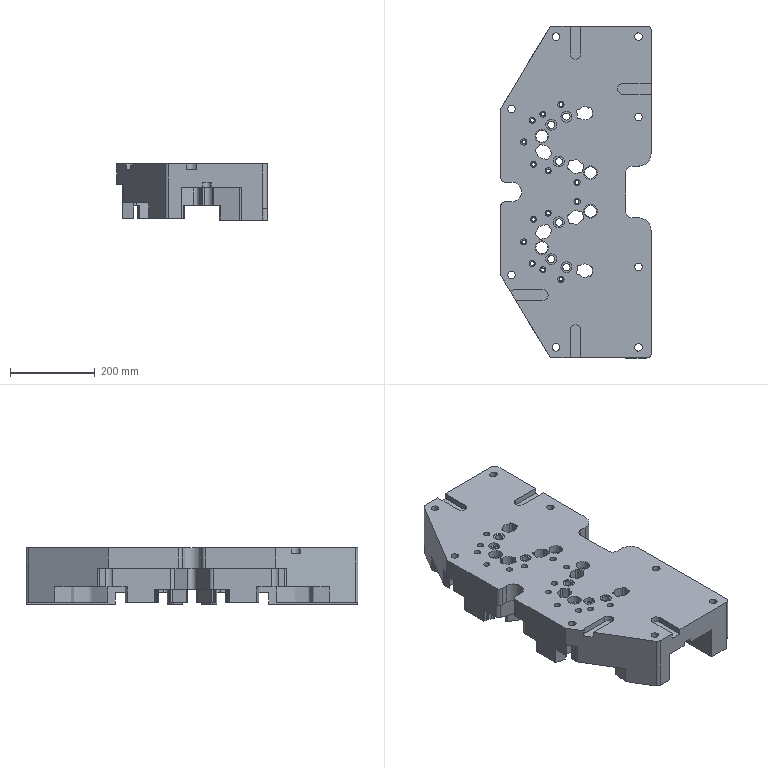Part | NX | features 7 2 | 1 solid | 487 faces | box 355 x 784 x 133 mm | volume 17502988 mm3 | plane 236 | cylinder 211 | cone 32 | spline 8 | commonest cylinder face diameters 20 x25 8 x24 10.3 x18 32 x16 9 x14 14.5 x14